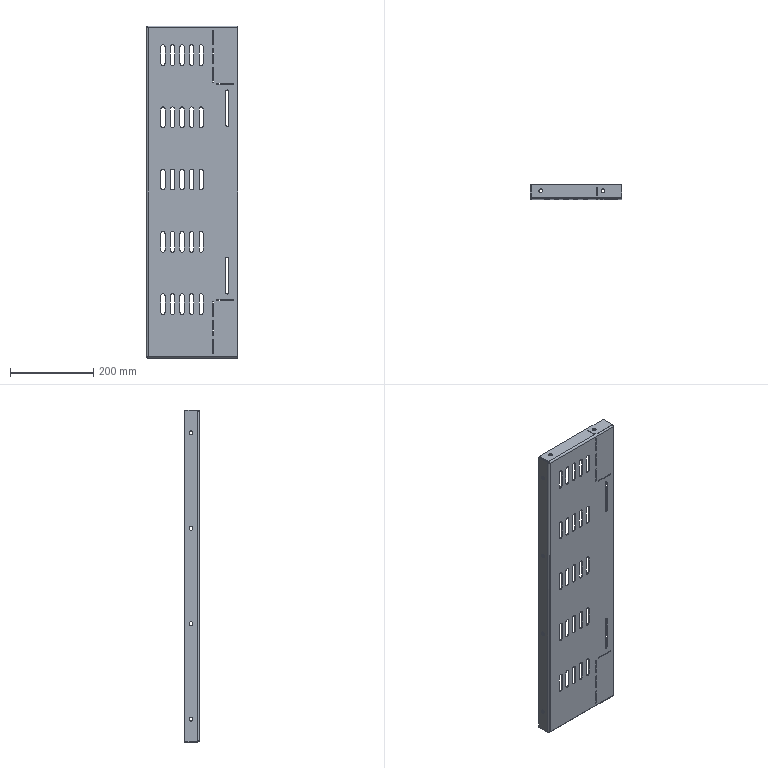Part | STEP file | 68352126 | 1 solid | 194 faces | box 220 x 35 x 800 mm | volume 401401 mm3 | plane 114 | cylinder 76 | spline 4 | commonest cylinder face diameters 10 x50 9 x16 7 x4 4 x3 8 x3